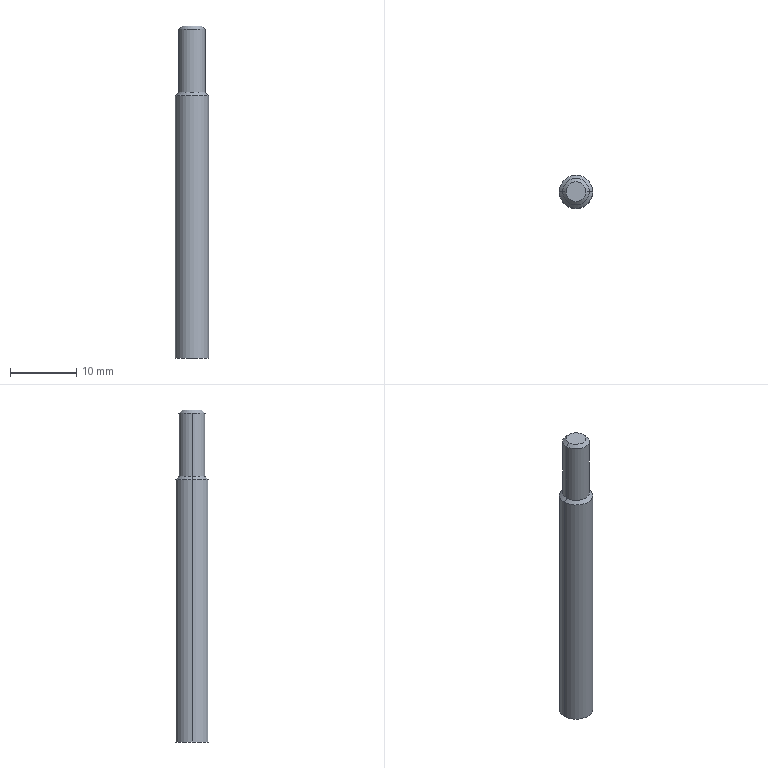Part | SolidWorks | features BaseBody 1 | 1 solid | 10 faces | box 5 x 5 x 50 mm | volume 907.789 mm3 | cylinder 4 | cone 4 | plane 2 | commonest cylinder face diameters 4 x2 5 x2
STEP:
#1=CARTESIAN_POINT('',(13.267,14.893,0.));
#2=VERTEX_POINT('',#1);
#3=CARTESIAN_POINT('',(8.267,14.893,0.));
#4=VERTEX_POINT('',#3);
#5=CARTESIAN_POINT('',(10.767,14.893,0.));
#6=DIRECTION('',(0.,0.,1.));
#7=DIRECTION('',(1.,0.,0.));
#8=AXIS2_PLACEMENT_3D('',#5,#6,#7);
#9=CIRCLE('',#8,2.5);
#10=EDGE_CURVE('',#2,#4,#9,.T.);
#11=ORIENTED_EDGE('',*,*,#10,.T.);
#12=CARTESIAN_POINT('',(8.267,14.893,39.5));
#13=VERTEX_POINT('',#12);
#14=CARTESIAN_POINT('',(8.267,14.893,0.));
#15=DIRECTION('',(0.,0.,1.));
#16=VECTOR('',#15,1000.);
#17=LINE('',#14,#16);
#18=EDGE_CURVE('',#4,#13,#17,.T.);
#19=ORIENTED_EDGE('',*,*,#18,.T.);
#20=CARTESIAN_POINT('',(13.267,14.893,39.5));
#21=VERTEX_POINT('',#20);
#22=CARTESIAN_POINT('',(10.767,14.893,39.5));
#23=DIRECTION('',(0.,0.,-1.));
#24=DIRECTION('',(1.,0.,0.));
#25=AXIS2_PLACEMENT_3D('',#22,#23,#24);
#26=CIRCLE('',#25,2.5);
#27=EDGE_CURVE('',#13,#21,#26,.T.);
#28=ORIENTED_EDGE('',*,*,#27,.T.);
#29=CARTESIAN_POINT('',(13.267,14.893,0.));
#30=DIRECTION('',(0.,0.,1.));
#31=VECTOR('',#30,1000.);
#32=LINE('',#29,#31);
#33=EDGE_CURVE('',#2,#21,#32,.T.);
#34=ORIENTED_EDGE('',*,*,#33,.F.);
#35=EDGE_LOOP('',(#11,#19,#28,#34));
#36=FACE_OUTER_BOUND('',#35,.T.);
#37=CARTESIAN_POINT('',(10.767,14.893,0.));
#38=DIRECTION('',(0.,0.,1.));
#39=DIRECTION('',(1.,0.,0.));
#40=AXIS2_PLACEMENT_3D('',#37,#38,#39);
#41=CYLINDRICAL_SURFACE('',#40,2.5);
#42=ADVANCED_FACE('',(#36),#41,.T.);
#43=CARTESIAN_POINT('',(8.767,14.893,40.));
#44=VERTEX_POINT('',#43);
#45=CARTESIAN_POINT('',(12.767,14.893,40.));
#46=VERTEX_POINT('',#45);
#47=CARTESIAN_POINT('',(10.767,14.893,40.));
#48=DIRECTION('',(0.,0.,-1.));
#49=DIRECTION('',(-1.,0.,0.));
#50=AXIS2_PLACEMENT_3D('',#47,#48,#49);
#51=CIRCLE('',#50,2.);
#52=EDGE_CURVE('',#44,#46,#51,.T.);
#53=ORIENTED_EDGE('',*,*,#52,.T.);
#54=CARTESIAN_POINT('',(13.267,14.893,39.5));
#55=DIRECTION('',(0.7071,0.,-0.7071));
#56=VECTOR('',#55,1000.);
#57=LINE('',#54,#56);
#58=EDGE_CURVE('',#46,#21,#57,.T.);
#59=ORIENTED_EDGE('',*,*,#58,.T.);
#60=ORIENTED_EDGE('',*,*,#27,.F.);
#61=CARTESIAN_POINT('',(8.267,14.893,39.5));
#62=DIRECTION('',(-0.7071,0.,-0.7071));
#63=VECTOR('',#62,1000.);
#64=LINE('',#61,#63);
#65=EDGE_CURVE('',#44,#13,#64,.T.);
#66=ORIENTED_EDGE('',*,*,#65,.F.);
#67=EDGE_LOOP('',(#53,#59,#60,#66));
#68=FACE_OUTER_BOUND('',#67,.T.);
#69=CARTESIAN_POINT('',(10.767,14.893,39.5));
#70=DIRECTION('',(0.,0.,-1.));
#71=DIRECTION('',(-1.,0.,0.));
#72=AXIS2_PLACEMENT_3D('',#69,#70,#71);
#73=CONICAL_SURFACE('',#72,2.5,0.7854);
#74=ADVANCED_FACE('',(#68),#73,.T.);
#75=CARTESIAN_POINT('',(8.767,14.893,49.5));
#76=VERTEX_POINT('',#75);
#77=CARTESIAN_POINT('',(12.767,14.893,49.5));
#78=VERTEX_POINT('',#77);
#79=CARTESIAN_POINT('',(10.767,14.893,49.5));
#80=DIRECTION('',(0.,0.,-1.));
#81=DIRECTION('',(-1.,0.,0.));
#82=AXIS2_PLACEMENT_3D('',#79,#80,#81);
#83=CIRCLE('',#82,2.);
#84=EDGE_CURVE('',#76,#78,#83,.T.);
#85=ORIENTED_EDGE('',*,*,#84,.T.);
#86=CARTESIAN_POINT('',(12.767,14.893,50.));
#87=DIRECTION('',(0.,0.,-1.));
#88=VECTOR('',#87,1000.);
#89=LINE('',#86,#88);
#90=EDGE_CURVE('',#78,#46,#89,.T.);
#91=ORIENTED_EDGE('',*,*,#90,.T.);
#92=ORIENTED_EDGE('',*,*,#52,.F.);
#93=CARTESIAN_POINT('',(8.767,14.893,50.));
#94=DIRECTION('',(0.,0.,-1.));
#95=VECTOR('',#94,1000.);
#96=LINE('',#93,#95);
#97=EDGE_CURVE('',#76,#44,#96,.T.);
#98=ORIENTED_EDGE('',*,*,#97,.F.);
#99=EDGE_LOOP('',(#85,#91,#92,#98));
#100=FACE_OUTER_BOUND('',#99,.T.);
#101=CARTESIAN_POINT('',(10.767,14.893,50.));
#102=DIRECTION('',(0.,0.,-1.));
#103=DIRECTION('',(-1.,0.,0.));
#104=AXIS2_PLACEMENT_3D('',#101,#102,#103);
#105=CYLINDRICAL_SURFACE('',#104,2.);
#106=ADVANCED_FACE('',(#100),#105,.T.);
#107=CARTESIAN_POINT('',(9.267,14.893,50.));
#108=VERTEX_POINT('',#107);
#109=CARTESIAN_POINT('',(12.267,14.893,50.));
#110=VERTEX_POINT('',#109);
#111=CARTESIAN_POINT('',(10.767,14.893,50.));
#112=DIRECTION('',(0.,0.,-1.));
#113=DIRECTION('',(-1.,0.,0.));
#114=AXIS2_PLACEMENT_3D('',#111,#112,#113);
#115=CIRCLE('',#114,1.5);
#116=EDGE_CURVE('',#108,#110,#115,.T.);
#117=ORIENTED_EDGE('',*,*,#116,.T.);
#118=CARTESIAN_POINT('',(12.767,14.893,49.5));
#119=DIRECTION('',(0.7071,0.,-0.7071));
#120=VECTOR('',#119,1000.);
#121=LINE('',#118,#120);
#122=EDGE_CURVE('',#110,#78,#121,.T.);
#123=ORIENTED_EDGE('',*,*,#122,.T.);
#124=ORIENTED_EDGE('',*,*,#84,.F.);
#125=CARTESIAN_POINT('',(8.767,14.893,49.5));
#126=DIRECTION('',(-0.7071,0.,-0.7071));
#127=VECTOR('',#126,1000.);
#128=LINE('',#125,#127);
#129=EDGE_CURVE('',#108,#76,#128,.T.);
#130=ORIENTED_EDGE('',*,*,#129,.F.);
#131=EDGE_LOOP('',(#117,#123,#124,#130));
#132=FACE_OUTER_BOUND('',#131,.T.);
#133=CARTESIAN_POINT('',(10.767,14.893,49.5));
#134=DIRECTION('',(0.,0.,-1.));
#135=DIRECTION('',(-1.,0.,0.));
#136=AXIS2_PLACEMENT_3D('',#133,#134,#135);
#137=CONICAL_SURFACE('',#136,2.,0.7854);
#138=ADVANCED_FACE('',(#132),#137,.T.);
#139=ORIENTED_EDGE('',*,*,#18,.F.);
#140=CARTESIAN_POINT('',(10.767,14.893,0.));
#141=DIRECTION('',(0.,0.,1.));
#142=DIRECTION('',(1.,0.,0.));
#143=AXIS2_PLACEMENT_3D('',#140,#141,#142);
#144=CIRCLE('',#143,2.5);
#145=EDGE_CURVE('',#4,#2,#144,.T.);
#146=ORIENTED_EDGE('',*,*,#145,.T.);
#147=ORIENTED_EDGE('',*,*,#33,.T.);
#148=CARTESIAN_POINT('',(10.767,14.893,39.5));
#149=DIRECTION('',(0.,0.,-1.));
#150=DIRECTION('',(1.,0.,0.));
#151=AXIS2_PLACEMENT_3D('',#148,#149,#150);
#152=CIRCLE('',#151,2.5);
#153=EDGE_CURVE('',#21,#13,#152,.T.);
#154=ORIENTED_EDGE('',*,*,#153,.T.);
#155=EDGE_LOOP('',(#139,#146,#147,#154));
#156=FACE_OUTER_BOUND('',#155,.T.);
#157=CARTESIAN_POINT('',(10.767,14.893,0.));
#158=DIRECTION('',(0.,0.,1.));
#159=DIRECTION('',(1.,0.,0.));
#160=AXIS2_PLACEMENT_3D('',#157,#158,#159);
#161=CYLINDRICAL_SURFACE('',#160,2.5);
#162=ADVANCED_FACE('',(#156),#161,.T.);
#163=ORIENTED_EDGE('',*,*,#58,.F.);
#164=CARTESIAN_POINT('',(10.767,14.893,40.));
#165=DIRECTION('',(0.,0.,-1.));
#166=DIRECTION('',(-1.,0.,0.));
#167=AXIS2_PLACEMENT_3D('',#164,#165,#166);
#168=CIRCLE('',#167,2.);
#169=EDGE_CURVE('',#46,#44,#168,.T.);
#170=ORIENTED_EDGE('',*,*,#169,.T.);
#171=ORIENTED_EDGE('',*,*,#65,.T.);
#172=ORIENTED_EDGE('',*,*,#153,.F.);
#173=EDGE_LOOP('',(#163,#170,#171,#172));
#174=FACE_OUTER_BOUND('',#173,.T.);
#175=CARTESIAN_POINT('',(10.767,14.893,39.5));
#176=DIRECTION('',(0.,0.,-1.));
#177=DIRECTION('',(-1.,0.,0.));
#178=AXIS2_PLACEMENT_3D('',#175,#176,#177);
#179=CONICAL_SURFACE('',#178,2.5,0.7854);
#180=ADVANCED_FACE('',(#174),#179,.T.);
#181=ORIENTED_EDGE('',*,*,#10,.F.);
#182=ORIENTED_EDGE('',*,*,#145,.F.);
#183=EDGE_LOOP('',(#181,#182));
#184=FACE_OUTER_BOUND('',#183,.T.);
#185=CARTESIAN_POINT('',(10.767,14.893,0.));
#186=DIRECTION('',(0.,0.,-1.));
#187=DIRECTION('',(-1.,0.,0.));
#188=AXIS2_PLACEMENT_3D('',#185,#186,#187);
#189=PLANE('',#188);
#190=ADVANCED_FACE('',(#184),#189,.T.);
#191=ORIENTED_EDGE('',*,*,#90,.F.);
#192=CARTESIAN_POINT('',(10.767,14.893,49.5));
#193=DIRECTION('',(0.,0.,-1.));
#194=DIRECTION('',(-1.,0.,0.));
#195=AXIS2_PLACEMENT_3D('',#192,#193,#194);
#196=CIRCLE('',#195,2.);
#197=EDGE_CURVE('',#78,#76,#196,.T.);
#198=ORIENTED_EDGE('',*,*,#197,.T.);
#199=ORIENTED_EDGE('',*,*,#97,.T.);
#200=ORIENTED_EDGE('',*,*,#169,.F.);
#201=EDGE_LOOP('',(#191,#198,#199,#200));
#202=FACE_OUTER_BOUND('',#201,.T.);
#203=CARTESIAN_POINT('',(10.767,14.893,50.));
#204=DIRECTION('',(0.,0.,-1.));
#205=DIRECTION('',(-1.,0.,0.));
#206=AXIS2_PLACEMENT_3D('',#203,#204,#205);
#207=CYLINDRICAL_SURFACE('',#206,2.);
#208=ADVANCED_FACE('',(#202),#207,.T.);
#209=ORIENTED_EDGE('',*,*,#122,.F.);
#210=CARTESIAN_POINT('',(10.767,14.893,50.));
#211=DIRECTION('',(0.,0.,-1.));
#212=DIRECTION('',(-1.,0.,0.));
#213=AXIS2_PLACEMENT_3D('',#210,#211,#212);
#214=CIRCLE('',#213,1.5);
#215=EDGE_CURVE('',#110,#108,#214,.T.);
#216=ORIENTED_EDGE('',*,*,#215,.T.);
#217=ORIENTED_EDGE('',*,*,#129,.T.);
#218=ORIENTED_EDGE('',*,*,#197,.F.);
#219=EDGE_LOOP('',(#209,#216,#217,#218));
#220=FACE_OUTER_BOUND('',#219,.T.);
#221=CARTESIAN_POINT('',(10.767,14.893,49.5));
#222=DIRECTION('',(0.,0.,-1.));
#223=DIRECTION('',(-1.,0.,0.));
#224=AXIS2_PLACEMENT_3D('',#221,#222,#223);
#225=CONICAL_SURFACE('',#224,2.,0.7854);
#226=ADVANCED_FACE('',(#220),#225,.T.);
#227=ORIENTED_EDGE('',*,*,#116,.F.);
#228=ORIENTED_EDGE('',*,*,#215,.F.);
#229=EDGE_LOOP('',(#227,#228));
#230=FACE_OUTER_BOUND('',#229,.T.);
#231=CARTESIAN_POINT('',(10.767,14.893,50.));
#232=DIRECTION('',(0.,0.,-1.));
#233=DIRECTION('',(-1.,0.,0.));
#234=AXIS2_PLACEMENT_3D('',#231,#232,#233);
#235=PLANE('',#234);
#236=ADVANCED_FACE('',(#230),#235,.F.);
#237=CLOSED_SHELL('',(#42,#74,#106,#138,#162,#180,#190,#208,#226,#236));
#238=MANIFOLD_SOLID_BREP('',#237);
#239=CARTESIAN_POINT('',(0.,0.,0.));
#240=DIRECTION('',(0.,0.,1.));
#241=DIRECTION('',(1.,0.,0.));
#242=AXIS2_PLACEMENT_3D('',#239,#240,#241);
#243=(LENGTH_UNIT()NAMED_UNIT(*)SI_UNIT(.MILLI.,.METRE.));
#244=UNCERTAINTY_MEASURE_WITH_UNIT(LENGTH_MEASURE(0.00001),#243,'','');
#245=(NAMED_UNIT(*)PLANE_ANGLE_UNIT()SI_UNIT($,.RADIAN.));
#246=(NAMED_UNIT(*)SI_UNIT($,.STERADIAN.)SOLID_ANGLE_UNIT());
#247=(GEOMETRIC_REPRESENTATION_CONTEXT(3)GLOBAL_UNCERTAINTY_ASSIGNED_CONTEXT((#244))GLOBAL_UNIT_ASSIGNED_CONTEXT((#243,#245,#246))REPRESENTATION_CONTEXT('',''));
#248=ADVANCED_BREP_SHAPE_REPRESENTATION('',(#238,#242),#247);